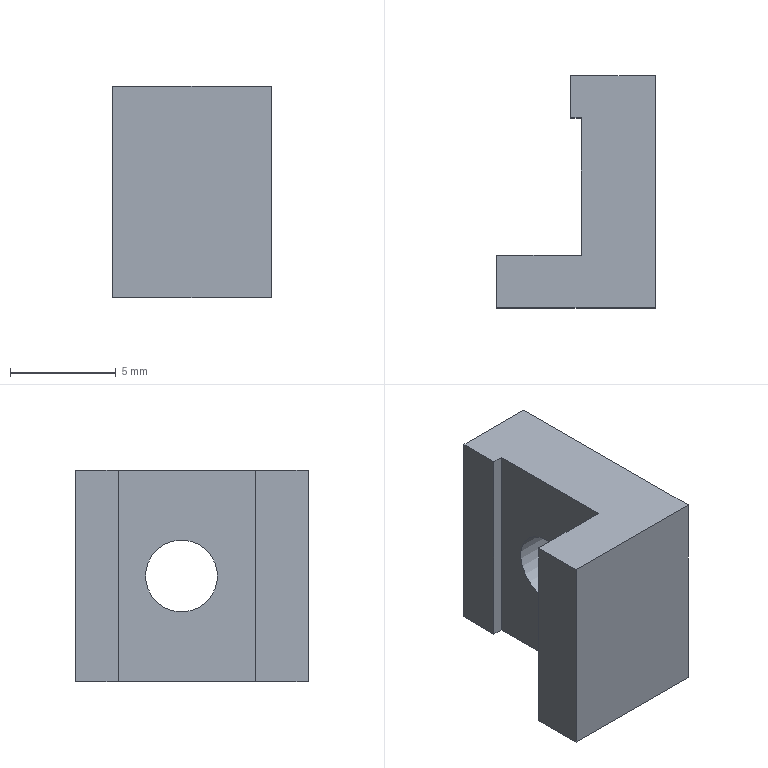Part | SolidWorks | features BaseBody 1 | 1 solid | 12 faces | box 7.5 x 11 x 10 mm | volume 463.223 mm3 | plane 10 | cylinder 2 | commonest cylinder face diameters 3.4 x2
STEP:
#1=CARTESIAN_POINT('',(-168.496,1830.044,8.7));
#2=VERTEX_POINT('',#1);
#3=CARTESIAN_POINT('',(-168.496,1830.044,5.3));
#4=VERTEX_POINT('',#3);
#5=CARTESIAN_POINT('',(-168.496,1830.044,7.));
#6=DIRECTION('',(1.,0.,0.));
#7=DIRECTION('',(0.,0.,-1.));
#8=AXIS2_PLACEMENT_3D('',#5,#6,#7);
#9=CIRCLE('',#8,1.7);
#10=EDGE_CURVE('',#2,#4,#9,.T.);
#11=ORIENTED_EDGE('',*,*,#10,.F.);
#12=CARTESIAN_POINT('',(-164.996,1830.044,8.7));
#13=VERTEX_POINT('',#12);
#14=CARTESIAN_POINT('',(-164.996,1830.044,8.7));
#15=DIRECTION('',(1.,0.,0.));
#16=VECTOR('',#15,1000.);
#17=LINE('',#14,#16);
#18=EDGE_CURVE('',#2,#13,#17,.T.);
#19=ORIENTED_EDGE('',*,*,#18,.T.);
#20=CARTESIAN_POINT('',(-164.996,1830.044,5.3));
#21=VERTEX_POINT('',#20);
#22=CARTESIAN_POINT('',(-164.996,1830.044,7.));
#23=DIRECTION('',(1.,0.,0.));
#24=DIRECTION('',(0.,0.,-1.));
#25=AXIS2_PLACEMENT_3D('',#22,#23,#24);
#26=CIRCLE('',#25,1.7);
#27=EDGE_CURVE('',#13,#21,#26,.T.);
#28=ORIENTED_EDGE('',*,*,#27,.T.);
#29=CARTESIAN_POINT('',(-164.996,1830.044,5.3));
#30=DIRECTION('',(1.,0.,0.));
#31=VECTOR('',#30,1000.);
#32=LINE('',#29,#31);
#33=EDGE_CURVE('',#4,#21,#32,.T.);
#34=ORIENTED_EDGE('',*,*,#33,.F.);
#35=EDGE_LOOP('',(#11,#19,#28,#34));
#36=FACE_OUTER_BOUND('',#35,.T.);
#37=CARTESIAN_POINT('',(-164.996,1830.044,7.));
#38=DIRECTION('',(1.,0.,0.));
#39=DIRECTION('',(0.,0.,-1.));
#40=AXIS2_PLACEMENT_3D('',#37,#38,#39);
#41=CYLINDRICAL_SURFACE('',#40,1.7);
#42=ADVANCED_FACE('',(#36),#41,.F.);
#43=CARTESIAN_POINT('',(-164.996,1830.044,7.));
#44=DIRECTION('',(1.,0.,0.));
#45=DIRECTION('',(0.,0.,-1.));
#46=AXIS2_PLACEMENT_3D('',#43,#44,#45);
#47=CIRCLE('',#46,1.7);
#48=EDGE_CURVE('',#21,#13,#47,.T.);
#49=ORIENTED_EDGE('',*,*,#48,.F.);
#50=ORIENTED_EDGE('',*,*,#27,.F.);
#51=EDGE_LOOP('',(#49,#50));
#52=FACE_BOUND('',#51,.T.);
#53=CARTESIAN_POINT('',(-164.996,1835.044,2.));
#54=VERTEX_POINT('',#53);
#55=CARTESIAN_POINT('',(-164.996,1824.044,2.));
#56=VERTEX_POINT('',#55);
#57=CARTESIAN_POINT('',(-164.996,1824.044,2.));
#58=DIRECTION('',(0.,-1.,0.));
#59=VECTOR('',#58,1000.);
#60=LINE('',#57,#59);
#61=EDGE_CURVE('',#54,#56,#60,.T.);
#62=ORIENTED_EDGE('',*,*,#61,.F.);
#63=CARTESIAN_POINT('',(-164.996,1835.044,12.));
#64=VERTEX_POINT('',#63);
#65=CARTESIAN_POINT('',(-164.996,1835.044,2.));
#66=DIRECTION('',(0.,0.,-1.));
#67=VECTOR('',#66,1000.);
#68=LINE('',#65,#67);
#69=EDGE_CURVE('',#64,#54,#68,.T.);
#70=ORIENTED_EDGE('',*,*,#69,.F.);
#71=CARTESIAN_POINT('',(-164.996,1824.044,12.));
#72=VERTEX_POINT('',#71);
#73=CARTESIAN_POINT('',(-164.996,1824.044,12.));
#74=DIRECTION('',(0.,1.,0.));
#75=VECTOR('',#74,1000.);
#76=LINE('',#73,#75);
#77=EDGE_CURVE('',#72,#64,#76,.T.);
#78=ORIENTED_EDGE('',*,*,#77,.F.);
#79=CARTESIAN_POINT('',(-164.996,1824.044,2.));
#80=DIRECTION('',(0.,0.,1.));
#81=VECTOR('',#80,1000.);
#82=LINE('',#79,#81);
#83=EDGE_CURVE('',#56,#72,#82,.T.);
#84=ORIENTED_EDGE('',*,*,#83,.F.);
#85=EDGE_LOOP('',(#62,#70,#78,#84));
#86=FACE_OUTER_BOUND('',#85,.T.);
#87=CARTESIAN_POINT('',(-164.996,1824.044,2.));
#88=DIRECTION('',(-1.,0.,0.));
#89=DIRECTION('',(0.,0.,1.));
#90=AXIS2_PLACEMENT_3D('',#87,#88,#89);
#91=PLANE('',#90);
#92=ADVANCED_FACE('',(#52,#86),#91,.F.);
#93=ORIENTED_EDGE('',*,*,#18,.F.);
#94=CARTESIAN_POINT('',(-168.496,1830.044,7.));
#95=DIRECTION('',(1.,0.,0.));
#96=DIRECTION('',(0.,0.,-1.));
#97=AXIS2_PLACEMENT_3D('',#94,#95,#96);
#98=CIRCLE('',#97,1.7);
#99=EDGE_CURVE('',#4,#2,#98,.T.);
#100=ORIENTED_EDGE('',*,*,#99,.F.);
#101=ORIENTED_EDGE('',*,*,#33,.T.);
#102=ORIENTED_EDGE('',*,*,#48,.T.);
#103=EDGE_LOOP('',(#93,#100,#101,#102));
#104=FACE_OUTER_BOUND('',#103,.T.);
#105=CARTESIAN_POINT('',(-164.996,1830.044,7.));
#106=DIRECTION('',(1.,0.,0.));
#107=DIRECTION('',(0.,0.,-1.));
#108=AXIS2_PLACEMENT_3D('',#105,#106,#107);
#109=CYLINDRICAL_SURFACE('',#108,1.7);
#110=ADVANCED_FACE('',(#104),#109,.F.);
#111=CARTESIAN_POINT('',(-172.496,1824.044,2.));
#112=VERTEX_POINT('',#111);
#113=CARTESIAN_POINT('',(-172.496,1824.044,2.));
#114=DIRECTION('',(-1.,0.,0.));
#115=VECTOR('',#114,1000.);
#116=LINE('',#113,#115);
#117=EDGE_CURVE('',#56,#112,#116,.T.);
#118=ORIENTED_EDGE('',*,*,#117,.F.);
#119=ORIENTED_EDGE('',*,*,#83,.T.);
#120=CARTESIAN_POINT('',(-172.496,1824.044,12.));
#121=VERTEX_POINT('',#120);
#122=CARTESIAN_POINT('',(-172.496,1824.044,12.));
#123=DIRECTION('',(1.,0.,0.));
#124=VECTOR('',#123,1000.);
#125=LINE('',#122,#124);
#126=EDGE_CURVE('',#121,#72,#125,.T.);
#127=ORIENTED_EDGE('',*,*,#126,.F.);
#128=CARTESIAN_POINT('',(-172.496,1824.044,2.));
#129=DIRECTION('',(0.,0.,1.));
#130=VECTOR('',#129,1000.);
#131=LINE('',#128,#130);
#132=EDGE_CURVE('',#112,#121,#131,.T.);
#133=ORIENTED_EDGE('',*,*,#132,.F.);
#134=EDGE_LOOP('',(#118,#119,#127,#133));
#135=FACE_OUTER_BOUND('',#134,.T.);
#136=CARTESIAN_POINT('',(-172.496,1824.044,2.));
#137=DIRECTION('',(0.,1.,0.));
#138=DIRECTION('',(0.,0.,1.));
#139=AXIS2_PLACEMENT_3D('',#136,#137,#138);
#140=PLANE('',#139);
#141=ADVANCED_FACE('',(#135),#140,.F.);
#142=CARTESIAN_POINT('',(-168.496,1833.044,2.));
#143=VERTEX_POINT('',#142);
#144=CARTESIAN_POINT('',(-168.496,1826.544,2.));
#145=VERTEX_POINT('',#144);
#146=CARTESIAN_POINT('',(-168.496,1824.044,2.));
#147=DIRECTION('',(0.,-1.,0.));
#148=VECTOR('',#147,1000.);
#149=LINE('',#146,#148);
#150=EDGE_CURVE('',#143,#145,#149,.T.);
#151=ORIENTED_EDGE('',*,*,#150,.F.);
#152=CARTESIAN_POINT('',(-168.996,1833.044,2.));
#153=VERTEX_POINT('',#152);
#154=CARTESIAN_POINT('',(-164.996,1833.044,2.));
#155=DIRECTION('',(1.,0.,0.));
#156=VECTOR('',#155,1000.);
#157=LINE('',#154,#156);
#158=EDGE_CURVE('',#153,#143,#157,.T.);
#159=ORIENTED_EDGE('',*,*,#158,.F.);
#160=CARTESIAN_POINT('',(-168.996,1835.044,2.));
#161=VERTEX_POINT('',#160);
#162=CARTESIAN_POINT('',(-168.996,1824.044,2.));
#163=DIRECTION('',(0.,-1.,0.));
#164=VECTOR('',#163,1000.);
#165=LINE('',#162,#164);
#166=EDGE_CURVE('',#161,#153,#165,.T.);
#167=ORIENTED_EDGE('',*,*,#166,.F.);
#168=CARTESIAN_POINT('',(-164.996,1835.044,2.));
#169=DIRECTION('',(-1.,0.,0.));
#170=VECTOR('',#169,1000.);
#171=LINE('',#168,#170);
#172=EDGE_CURVE('',#54,#161,#171,.T.);
#173=ORIENTED_EDGE('',*,*,#172,.F.);
#174=ORIENTED_EDGE('',*,*,#61,.T.);
#175=ORIENTED_EDGE('',*,*,#117,.T.);
#176=CARTESIAN_POINT('',(-172.496,1826.544,2.));
#177=VERTEX_POINT('',#176);
#178=CARTESIAN_POINT('',(-172.496,1824.044,2.));
#179=DIRECTION('',(0.,-1.,0.));
#180=VECTOR('',#179,1000.);
#181=LINE('',#178,#180);
#182=EDGE_CURVE('',#177,#112,#181,.T.);
#183=ORIENTED_EDGE('',*,*,#182,.F.);
#184=CARTESIAN_POINT('',(-164.996,1826.544,2.));
#185=DIRECTION('',(-1.,0.,0.));
#186=VECTOR('',#185,1000.);
#187=LINE('',#184,#186);
#188=EDGE_CURVE('',#145,#177,#187,.T.);
#189=ORIENTED_EDGE('',*,*,#188,.F.);
#190=EDGE_LOOP('',(#151,#159,#167,#173,#174,#175,#183,#189));
#191=FACE_OUTER_BOUND('',#190,.T.);
#192=CARTESIAN_POINT('',(-164.996,1824.044,2.));
#193=DIRECTION('',(0.,0.,1.));
#194=DIRECTION('',(1.,0.,0.));
#195=AXIS2_PLACEMENT_3D('',#192,#193,#194);
#196=PLANE('',#195);
#197=ADVANCED_FACE('',(#191),#196,.F.);
#198=ORIENTED_EDGE('',*,*,#172,.T.);
#199=CARTESIAN_POINT('',(-168.996,1835.044,12.));
#200=VERTEX_POINT('',#199);
#201=CARTESIAN_POINT('',(-168.996,1835.044,2.));
#202=DIRECTION('',(0.,0.,-1.));
#203=VECTOR('',#202,1000.);
#204=LINE('',#201,#203);
#205=EDGE_CURVE('',#200,#161,#204,.T.);
#206=ORIENTED_EDGE('',*,*,#205,.F.);
#207=CARTESIAN_POINT('',(-164.996,1835.044,12.));
#208=DIRECTION('',(-1.,0.,0.));
#209=VECTOR('',#208,1000.);
#210=LINE('',#207,#209);
#211=EDGE_CURVE('',#64,#200,#210,.T.);
#212=ORIENTED_EDGE('',*,*,#211,.F.);
#213=ORIENTED_EDGE('',*,*,#69,.T.);
#214=EDGE_LOOP('',(#198,#206,#212,#213));
#215=FACE_OUTER_BOUND('',#214,.T.);
#216=CARTESIAN_POINT('',(-164.996,1835.044,2.));
#217=DIRECTION('',(0.,-1.,0.));
#218=DIRECTION('',(0.,0.,-1.));
#219=AXIS2_PLACEMENT_3D('',#216,#217,#218);
#220=PLANE('',#219);
#221=ADVANCED_FACE('',(#215),#220,.F.);
#222=CARTESIAN_POINT('',(-168.496,1826.544,12.));
#223=VERTEX_POINT('',#222);
#224=CARTESIAN_POINT('',(-172.496,1826.544,12.));
#225=VERTEX_POINT('',#224);
#226=CARTESIAN_POINT('',(-164.996,1826.544,12.));
#227=DIRECTION('',(-1.,0.,0.));
#228=VECTOR('',#227,1000.);
#229=LINE('',#226,#228);
#230=EDGE_CURVE('',#223,#225,#229,.T.);
#231=ORIENTED_EDGE('',*,*,#230,.T.);
#232=CARTESIAN_POINT('',(-172.496,1824.044,12.));
#233=DIRECTION('',(0.,-1.,0.));
#234=VECTOR('',#233,1000.);
#235=LINE('',#232,#234);
#236=EDGE_CURVE('',#225,#121,#235,.T.);
#237=ORIENTED_EDGE('',*,*,#236,.T.);
#238=ORIENTED_EDGE('',*,*,#126,.T.);
#239=ORIENTED_EDGE('',*,*,#77,.T.);
#240=ORIENTED_EDGE('',*,*,#211,.T.);
#241=CARTESIAN_POINT('',(-168.996,1833.044,12.));
#242=VERTEX_POINT('',#241);
#243=CARTESIAN_POINT('',(-168.996,1824.044,12.));
#244=DIRECTION('',(0.,-1.,0.));
#245=VECTOR('',#244,1000.);
#246=LINE('',#243,#245);
#247=EDGE_CURVE('',#200,#242,#246,.T.);
#248=ORIENTED_EDGE('',*,*,#247,.T.);
#249=CARTESIAN_POINT('',(-168.496,1833.044,12.));
#250=VERTEX_POINT('',#249);
#251=CARTESIAN_POINT('',(-164.996,1833.044,12.));
#252=DIRECTION('',(1.,0.,0.));
#253=VECTOR('',#252,1000.);
#254=LINE('',#251,#253);
#255=EDGE_CURVE('',#242,#250,#254,.T.);
#256=ORIENTED_EDGE('',*,*,#255,.T.);
#257=CARTESIAN_POINT('',(-168.496,1824.044,12.));
#258=DIRECTION('',(0.,-1.,0.));
#259=VECTOR('',#258,1000.);
#260=LINE('',#257,#259);
#261=EDGE_CURVE('',#250,#223,#260,.T.);
#262=ORIENTED_EDGE('',*,*,#261,.T.);
#263=EDGE_LOOP('',(#231,#237,#238,#239,#240,#248,#256,#262));
#264=FACE_OUTER_BOUND('',#263,.T.);
#265=CARTESIAN_POINT('',(-164.996,1824.044,12.));
#266=DIRECTION('',(0.,0.,1.));
#267=DIRECTION('',(1.,0.,0.));
#268=AXIS2_PLACEMENT_3D('',#265,#266,#267);
#269=PLANE('',#268);
#270=ADVANCED_FACE('',(#264),#269,.T.);
#271=ORIENTED_EDGE('',*,*,#99,.T.);
#272=ORIENTED_EDGE('',*,*,#10,.T.);
#273=EDGE_LOOP('',(#271,#272));
#274=FACE_BOUND('',#273,.T.);
#275=ORIENTED_EDGE('',*,*,#150,.T.);
#276=CARTESIAN_POINT('',(-168.496,1826.544,2.));
#277=DIRECTION('',(0.,0.,-1.));
#278=VECTOR('',#277,1000.);
#279=LINE('',#276,#278);
#280=EDGE_CURVE('',#223,#145,#279,.T.);
#281=ORIENTED_EDGE('',*,*,#280,.F.);
#282=ORIENTED_EDGE('',*,*,#261,.F.);
#283=CARTESIAN_POINT('',(-168.496,1833.044,2.));
#284=DIRECTION('',(0.,0.,1.));
#285=VECTOR('',#284,1000.);
#286=LINE('',#283,#285);
#287=EDGE_CURVE('',#143,#250,#286,.T.);
#288=ORIENTED_EDGE('',*,*,#287,.F.);
#289=EDGE_LOOP('',(#275,#281,#282,#288));
#290=FACE_OUTER_BOUND('',#289,.T.);
#291=CARTESIAN_POINT('',(-168.496,1833.044,2.));
#292=DIRECTION('',(1.,0.,0.));
#293=DIRECTION('',(0.,0.,-1.));
#294=AXIS2_PLACEMENT_3D('',#291,#292,#293);
#295=PLANE('',#294);
#296=ADVANCED_FACE('',(#274,#290),#295,.F.);
#297=ORIENTED_EDGE('',*,*,#182,.T.);
#298=ORIENTED_EDGE('',*,*,#132,.T.);
#299=ORIENTED_EDGE('',*,*,#236,.F.);
#300=CARTESIAN_POINT('',(-172.496,1826.544,2.));
#301=DIRECTION('',(0.,0.,1.));
#302=VECTOR('',#301,1000.);
#303=LINE('',#300,#302);
#304=EDGE_CURVE('',#177,#225,#303,.T.);
#305=ORIENTED_EDGE('',*,*,#304,.F.);
#306=EDGE_LOOP('',(#297,#298,#299,#305));
#307=FACE_OUTER_BOUND('',#306,.T.);
#308=CARTESIAN_POINT('',(-172.496,1826.544,2.));
#309=DIRECTION('',(1.,0.,0.));
#310=DIRECTION('',(0.,0.,-1.));
#311=AXIS2_PLACEMENT_3D('',#308,#309,#310);
#312=PLANE('',#311);
#313=ADVANCED_FACE('',(#307),#312,.F.);
#314=ORIENTED_EDGE('',*,*,#188,.T.);
#315=ORIENTED_EDGE('',*,*,#304,.T.);
#316=ORIENTED_EDGE('',*,*,#230,.F.);
#317=ORIENTED_EDGE('',*,*,#280,.T.);
#318=EDGE_LOOP('',(#314,#315,#316,#317));
#319=FACE_OUTER_BOUND('',#318,.T.);
#320=CARTESIAN_POINT('',(-168.496,1826.544,2.));
#321=DIRECTION('',(0.,-1.,0.));
#322=DIRECTION('',(0.,0.,-1.));
#323=AXIS2_PLACEMENT_3D('',#320,#321,#322);
#324=PLANE('',#323);
#325=ADVANCED_FACE('',(#319),#324,.F.);
#326=ORIENTED_EDGE('',*,*,#158,.T.);
#327=ORIENTED_EDGE('',*,*,#287,.T.);
#328=ORIENTED_EDGE('',*,*,#255,.F.);
#329=CARTESIAN_POINT('',(-168.996,1833.044,2.));
#330=DIRECTION('',(0.,0.,1.));
#331=VECTOR('',#330,1000.);
#332=LINE('',#329,#331);
#333=EDGE_CURVE('',#153,#242,#332,.T.);
#334=ORIENTED_EDGE('',*,*,#333,.F.);
#335=EDGE_LOOP('',(#326,#327,#328,#334));
#336=FACE_OUTER_BOUND('',#335,.T.);
#337=CARTESIAN_POINT('',(-168.996,1833.044,2.));
#338=DIRECTION('',(0.,1.,0.));
#339=DIRECTION('',(0.,0.,1.));
#340=AXIS2_PLACEMENT_3D('',#337,#338,#339);
#341=PLANE('',#340);
#342=ADVANCED_FACE('',(#336),#341,.F.);
#343=ORIENTED_EDGE('',*,*,#166,.T.);
#344=ORIENTED_EDGE('',*,*,#333,.T.);
#345=ORIENTED_EDGE('',*,*,#247,.F.);
#346=ORIENTED_EDGE('',*,*,#205,.T.);
#347=EDGE_LOOP('',(#343,#344,#345,#346));
#348=FACE_OUTER_BOUND('',#347,.T.);
#349=CARTESIAN_POINT('',(-168.996,1835.044,2.));
#350=DIRECTION('',(1.,0.,0.));
#351=DIRECTION('',(0.,0.,-1.));
#352=AXIS2_PLACEMENT_3D('',#349,#350,#351);
#353=PLANE('',#352);
#354=ADVANCED_FACE('',(#348),#353,.F.);
#355=CLOSED_SHELL('',(#42,#92,#110,#141,#197,#221,#270,#296,#313,#325,#342,#354));
#356=MANIFOLD_SOLID_BREP('',#355);
#357=CARTESIAN_POINT('',(0.,0.,0.));
#358=DIRECTION('',(0.,0.,1.));
#359=DIRECTION('',(1.,0.,0.));
#360=AXIS2_PLACEMENT_3D('',#357,#358,#359);
#361=(LENGTH_UNIT()NAMED_UNIT(*)SI_UNIT(.MILLI.,.METRE.));
#362=UNCERTAINTY_MEASURE_WITH_UNIT(LENGTH_MEASURE(0.00001),#361,'','');
#363=(NAMED_UNIT(*)PLANE_ANGLE_UNIT()SI_UNIT($,.RADIAN.));
#364=(NAMED_UNIT(*)SI_UNIT($,.STERADIAN.)SOLID_ANGLE_UNIT());
#365=(GEOMETRIC_REPRESENTATION_CONTEXT(3)GLOBAL_UNCERTAINTY_ASSIGNED_CONTEXT((#362))GLOBAL_UNIT_ASSIGNED_CONTEXT((#361,#363,#364))REPRESENTATION_CONTEXT('',''));
#366=ADVANCED_BREP_SHAPE_REPRESENTATION('',(#356,#360),#365);